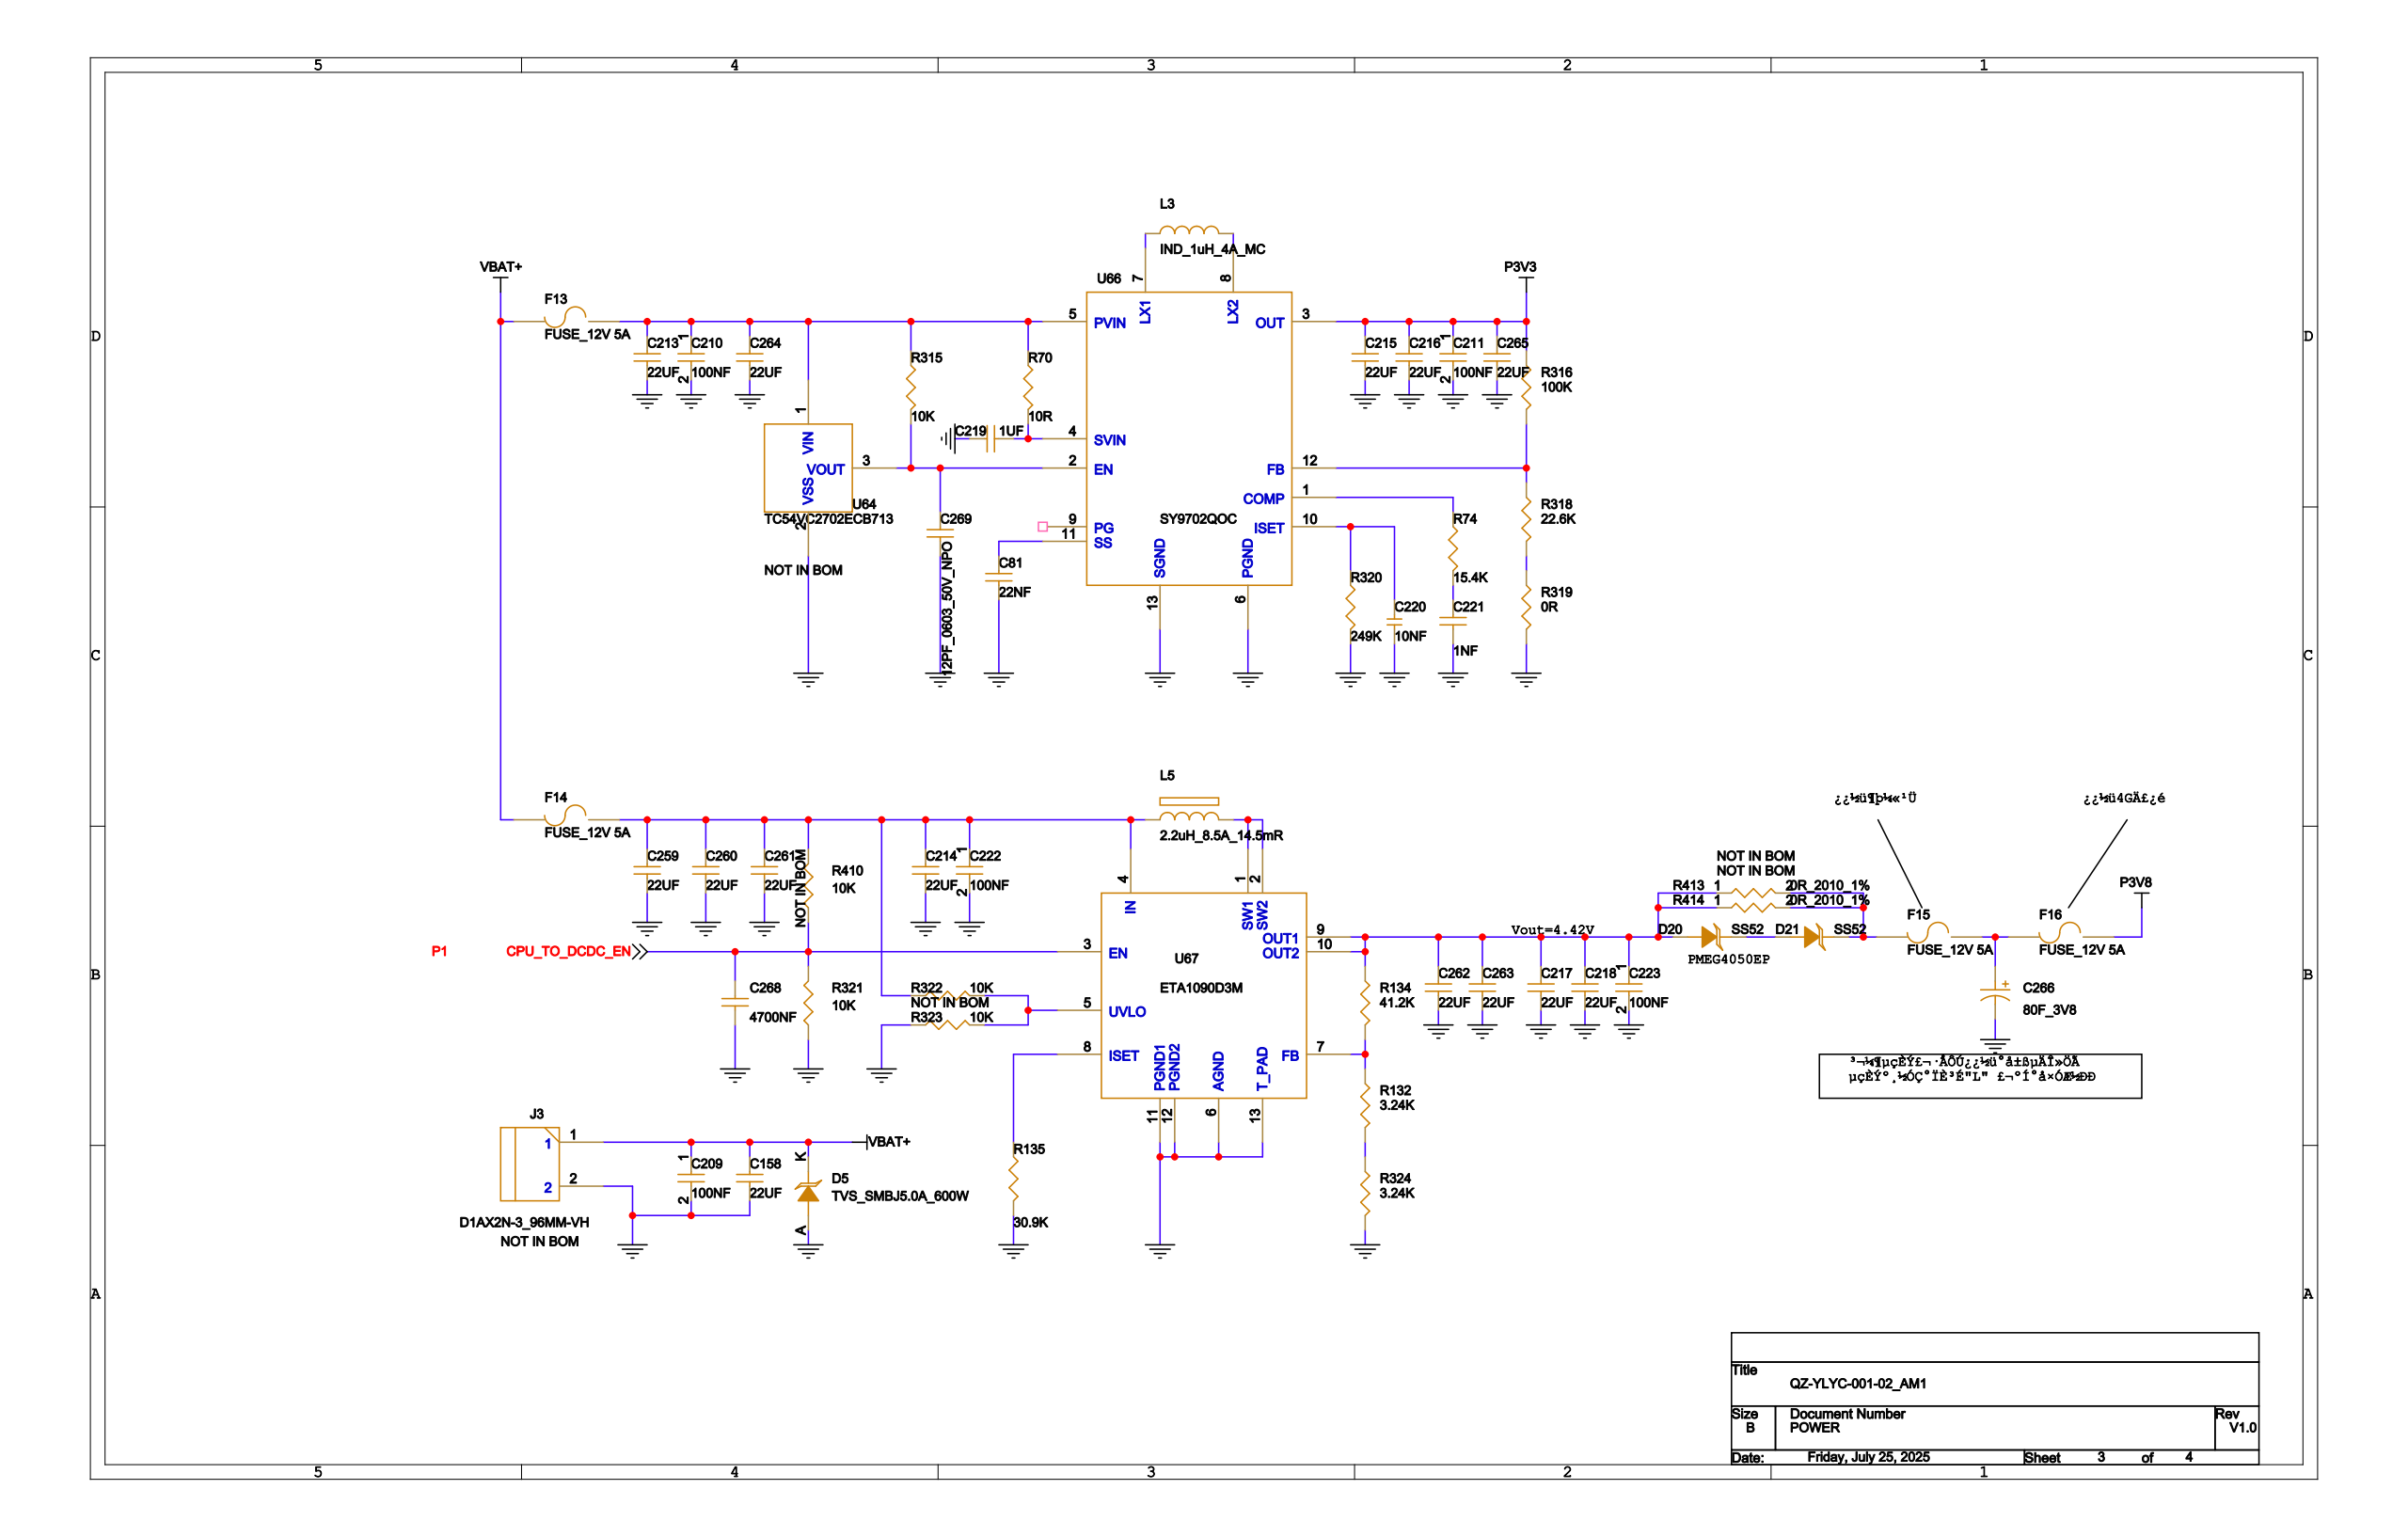Circuit board | Cadence Allegro | 366 parts | 230 nets | one sheet of the schematic
Parts on this sheet (reference | value | footprint):
C81 | C0603
C158 | C1206
C209 | C0603
C210 | C0603
C211 | C0603
C213 | C1206
C214 | C1206
C215 | C1206
C216 | C1206
C217 | C1206
C218 | C1206
C219 | C0603
C220 | C0603
C221 | C0603
C222 | C0603
C223 | C0603
C259 | C1206
C260 | C1206
C261 | C1206
C262 | C1206
C263 | C1206
C264 | C1206
C265 | C1206
C266 | DE10MM
C268 | C0603
C269 | C0603
D5 | SMA
D20 | SMB
D21 | SMB
F13 | FUSE_798X544
F14 | FUSE_798X544
F15 | FUSE_798X544
F16 | FUSE_798X544
J3 | D1AX2N-3_96MM-VH
L3 | L-4X4-IND_1UH_4A_MC
L5 | IND_4R7UH_10A5
R70 | R1206
R74 | R0603
R132 | R0603
R134 | R0603
R135 | R0603
R315 | R0603
R316 | R0603
R318 | R0603
R319 | R0603
R320 | R0603
R321 | R0603
R322 | R0603
R323 | R0603
R324 | R0603
R410 | R0603
R413 | R2010
R414 | R2010
U64 | SOT-23A-3
U66 | QFN2X3-13
U67 | DFN3X3_12
Nets of these parts (net: part-pin ...):
P3V8: F16-1
N613607: C266-1 F15-1 F16-2
N121950: C210-1 C213-1 C264-1 F13-1 R70-1 R315-1 U64-1 U66-5
VBAT+: C158-1 C209-1 D5-K F13-2 F14-2 J3-1
N122508: C214-1 C222-1 C259-1 C260-1 C261-1 F14-1 L5-1 R322-1 R410-2 U67-4
N606141: D21-K F15-2 R413-2 R414-2
N121868: L3-1 U66-7
N121872: L3-2 U66-8
N122532: L5-2 U67-1 U67-2
N122810: R132-1 R134-2 U67-7
N122858: R132-2 R324-1
GND: C81-2 C158-2 C209-2 C210-2 C211-2 C213-2 C214-2 C215-2 C216-2 C217-2 C218-2 C219-1 C220-1 C221-2 C222-2 C223-2 C259-2 C260-2 C261-2 C262-2 C263-2 C264-2 C265-2 C266-2 C268-2 C269-2 D5-A J3-2 R135-2 R319-2 R320-2 R321-1 R323-1 R324-2 U64-2 U66-6 U66-13 U67-6 U67-11 U67-12 U67-13
N122814: R135-1 U67-8
N122674: C217-1 C218-1 C223-1 C262-1 C263-1 D20-A R134-1 R413-1 R414-1 U67-9 U67-10
P3V3: C211-1 C215-1 C216-1 C265-1 R316-1 U66-3
N606157: D20-K D21-A
CPU_TO_DCDC_EN: C268-1 R321-2 R410-1 U67-3
N273444: R322-2 R323-2 U67-5
N122232: C219-2 R70-2 U66-4
N122208: C269-1 R315-2 U64-3 U66-2
N122296: C220-2 R320-1 U66-10
N122372: C221-1 R74-2
N122324: C81-1 U66-11
N122336: R318-2 R319-1
N122236: R316-2 R318-1 U66-12
N122272: R74-1 U66-1